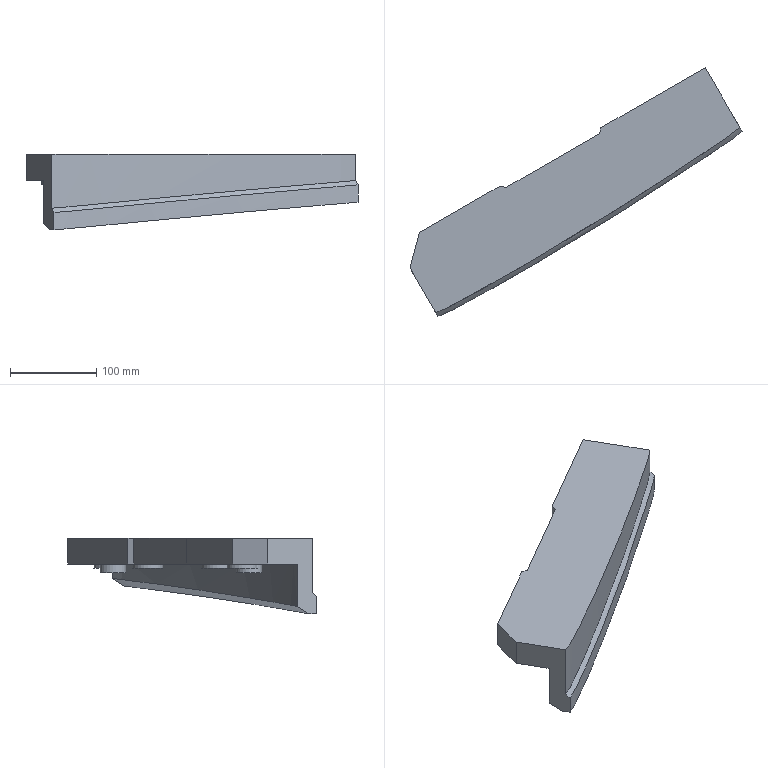Part | NX | features solid 2 | 1 solid | 28 faces | box 384.668 x 288.238 x 87.73 mm | volume 1479776 mm3 | plane 15 | spline 7 | cylinder 6 | commonest cylinder face diameters 35 x4 30 x2